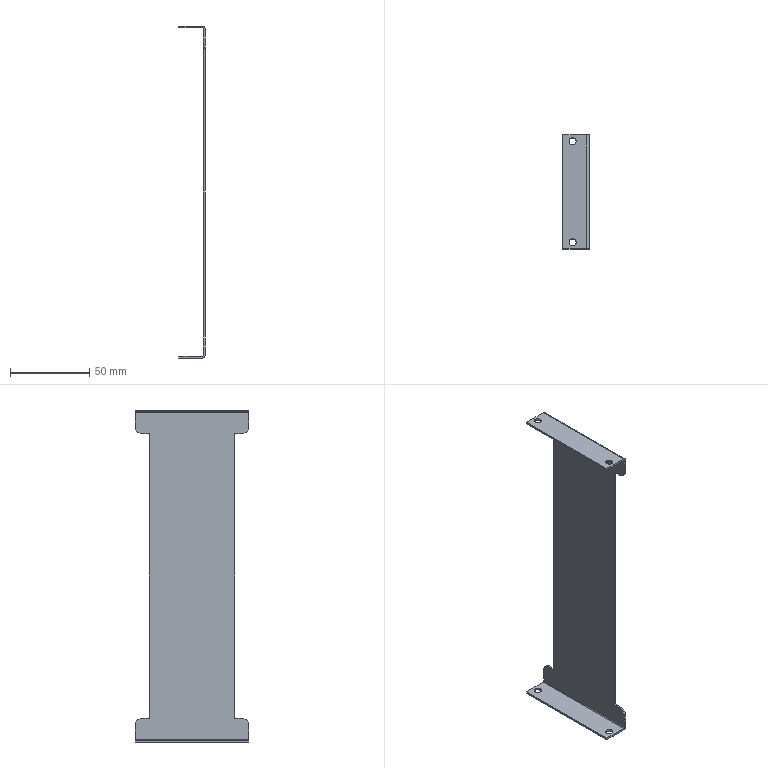Part | STEP file | 复件 FFH80-GY-007^复件 FFH85-B3 -02_三轴模组 | 1 solid | 34 faces | box 16.7 x 71.8 x 210 mm | volume 16698 mm3 | plane 18 | cylinder 16 | commonest cylinder face diameters 4.5 x8 8 x4 1 x2 3.4 x2
STEP:
#1=CARTESIAN_POINT('',(-12.75,-32.,102.6));
#2=VERTEX_POINT('',#1);
#3=CARTESIAN_POINT('',(-8.25,-32.,102.6));
#4=VERTEX_POINT('',#3);
#5=CARTESIAN_POINT('',(-10.5,-32.,102.6));
#6=DIRECTION('',(0.,0.,1.));
#7=DIRECTION('',(1.,0.,0.));
#8=AXIS2_PLACEMENT_3D('',#5,#6,#7);
#9=CIRCLE('',#8,2.25);
#10=EDGE_CURVE('',#2,#4,#9,.T.);
#11=ORIENTED_EDGE('',*,*,#10,.F.);
#12=CARTESIAN_POINT('',(-12.75,-32.,103.8));
#13=VERTEX_POINT('',#12);
#14=CARTESIAN_POINT('',(-12.75,-32.,-106.2));
#15=DIRECTION('',(0.,0.,1.));
#16=VECTOR('',#15,1000.);
#17=LINE('',#14,#16);
#18=EDGE_CURVE('',#2,#13,#17,.T.);
#19=ORIENTED_EDGE('',*,*,#18,.T.);
#20=CARTESIAN_POINT('',(-8.25,-32.,103.8));
#21=VERTEX_POINT('',#20);
#22=CARTESIAN_POINT('',(-10.5,-32.,103.8));
#23=DIRECTION('',(0.,0.,1.));
#24=DIRECTION('',(1.,0.,0.));
#25=AXIS2_PLACEMENT_3D('',#22,#23,#24);
#26=CIRCLE('',#25,2.25);
#27=EDGE_CURVE('',#13,#21,#26,.T.);
#28=ORIENTED_EDGE('',*,*,#27,.T.);
#29=CARTESIAN_POINT('',(-8.25,-32.,-106.2));
#30=DIRECTION('',(0.,0.,1.));
#31=VECTOR('',#30,1000.);
#32=LINE('',#29,#31);
#33=EDGE_CURVE('',#4,#21,#32,.T.);
#34=ORIENTED_EDGE('',*,*,#33,.F.);
#35=EDGE_LOOP('',(#11,#19,#28,#34));
#36=FACE_OUTER_BOUND('',#35,.T.);
#37=CARTESIAN_POINT('',(-10.5,-32.,-106.2));
#38=DIRECTION('',(0.,0.,1.));
#39=DIRECTION('',(1.,0.,0.));
#40=AXIS2_PLACEMENT_3D('',#37,#38,#39);
#41=CYLINDRICAL_SURFACE('',#40,2.25);
#42=ADVANCED_FACE('',(#36),#41,.F.);
#43=CARTESIAN_POINT('',(-12.75,32.,102.6));
#44=VERTEX_POINT('',#43);
#45=CARTESIAN_POINT('',(-8.25,32.,102.6));
#46=VERTEX_POINT('',#45);
#47=CARTESIAN_POINT('',(-10.5,32.,102.6));
#48=DIRECTION('',(0.,0.,1.));
#49=DIRECTION('',(1.,0.,0.));
#50=AXIS2_PLACEMENT_3D('',#47,#48,#49);
#51=CIRCLE('',#50,2.25);
#52=EDGE_CURVE('',#44,#46,#51,.T.);
#53=ORIENTED_EDGE('',*,*,#52,.F.);
#54=CARTESIAN_POINT('',(-12.75,32.,103.8));
#55=VERTEX_POINT('',#54);
#56=CARTESIAN_POINT('',(-12.75,32.,-106.2));
#57=DIRECTION('',(0.,0.,1.));
#58=VECTOR('',#57,1000.);
#59=LINE('',#56,#58);
#60=EDGE_CURVE('',#44,#55,#59,.T.);
#61=ORIENTED_EDGE('',*,*,#60,.T.);
#62=CARTESIAN_POINT('',(-8.25,32.,103.8));
#63=VERTEX_POINT('',#62);
#64=CARTESIAN_POINT('',(-10.5,32.,103.8));
#65=DIRECTION('',(0.,0.,1.));
#66=DIRECTION('',(1.,0.,0.));
#67=AXIS2_PLACEMENT_3D('',#64,#65,#66);
#68=CIRCLE('',#67,2.25);
#69=EDGE_CURVE('',#55,#63,#68,.T.);
#70=ORIENTED_EDGE('',*,*,#69,.T.);
#71=CARTESIAN_POINT('',(-8.25,32.,-106.2));
#72=DIRECTION('',(0.,0.,1.));
#73=VECTOR('',#72,1000.);
#74=LINE('',#71,#73);
#75=EDGE_CURVE('',#46,#63,#74,.T.);
#76=ORIENTED_EDGE('',*,*,#75,.F.);
#77=EDGE_LOOP('',(#53,#61,#70,#76));
#78=FACE_OUTER_BOUND('',#77,.T.);
#79=CARTESIAN_POINT('',(-10.5,32.,-106.2));
#80=DIRECTION('',(0.,0.,1.));
#81=DIRECTION('',(1.,0.,0.));
#82=AXIS2_PLACEMENT_3D('',#79,#80,#81);
#83=CYLINDRICAL_SURFACE('',#82,2.25);
#84=ADVANCED_FACE('',(#78),#83,.F.);
#85=CARTESIAN_POINT('',(-8.25,-32.,-106.2));
#86=VERTEX_POINT('',#85);
#87=CARTESIAN_POINT('',(-12.75,-32.,-106.2));
#88=VERTEX_POINT('',#87);
#89=CARTESIAN_POINT('',(-10.5,-32.,-106.2));
#90=DIRECTION('',(0.,0.,-1.));
#91=DIRECTION('',(1.,0.,0.));
#92=AXIS2_PLACEMENT_3D('',#89,#90,#91);
#93=CIRCLE('',#92,2.25);
#94=EDGE_CURVE('',#86,#88,#93,.T.);
#95=ORIENTED_EDGE('',*,*,#94,.T.);
#96=CARTESIAN_POINT('',(-12.75,-32.,-105.));
#97=VERTEX_POINT('',#96);
#98=CARTESIAN_POINT('',(-12.75,-32.,-106.2));
#99=DIRECTION('',(0.,0.,1.));
#100=VECTOR('',#99,1000.);
#101=LINE('',#98,#100);
#102=EDGE_CURVE('',#88,#97,#101,.T.);
#103=ORIENTED_EDGE('',*,*,#102,.T.);
#104=CARTESIAN_POINT('',(-8.25,-32.,-105.));
#105=VERTEX_POINT('',#104);
#106=CARTESIAN_POINT('',(-10.5,-32.,-105.));
#107=DIRECTION('',(0.,0.,-1.));
#108=DIRECTION('',(1.,0.,0.));
#109=AXIS2_PLACEMENT_3D('',#106,#107,#108);
#110=CIRCLE('',#109,2.25);
#111=EDGE_CURVE('',#105,#97,#110,.T.);
#112=ORIENTED_EDGE('',*,*,#111,.F.);
#113=CARTESIAN_POINT('',(-8.25,-32.,-106.2));
#114=DIRECTION('',(0.,0.,1.));
#115=VECTOR('',#114,1000.);
#116=LINE('',#113,#115);
#117=EDGE_CURVE('',#86,#105,#116,.T.);
#118=ORIENTED_EDGE('',*,*,#117,.F.);
#119=EDGE_LOOP('',(#95,#103,#112,#118));
#120=FACE_OUTER_BOUND('',#119,.T.);
#121=CARTESIAN_POINT('',(-10.5,-32.,-106.2));
#122=DIRECTION('',(0.,0.,1.));
#123=DIRECTION('',(1.,0.,0.));
#124=AXIS2_PLACEMENT_3D('',#121,#122,#123);
#125=CYLINDRICAL_SURFACE('',#124,2.25);
#126=ADVANCED_FACE('',(#120),#125,.F.);
#127=CARTESIAN_POINT('',(-8.25,32.,-106.2));
#128=VERTEX_POINT('',#127);
#129=CARTESIAN_POINT('',(-12.75,32.,-106.2));
#130=VERTEX_POINT('',#129);
#131=CARTESIAN_POINT('',(-10.5,32.,-106.2));
#132=DIRECTION('',(0.,0.,-1.));
#133=DIRECTION('',(1.,0.,0.));
#134=AXIS2_PLACEMENT_3D('',#131,#132,#133);
#135=CIRCLE('',#134,2.25);
#136=EDGE_CURVE('',#128,#130,#135,.T.);
#137=ORIENTED_EDGE('',*,*,#136,.T.);
#138=CARTESIAN_POINT('',(-12.75,32.,-105.));
#139=VERTEX_POINT('',#138);
#140=CARTESIAN_POINT('',(-12.75,32.,-106.2));
#141=DIRECTION('',(0.,0.,1.));
#142=VECTOR('',#141,1000.);
#143=LINE('',#140,#142);
#144=EDGE_CURVE('',#130,#139,#143,.T.);
#145=ORIENTED_EDGE('',*,*,#144,.T.);
#146=CARTESIAN_POINT('',(-8.25,32.,-105.));
#147=VERTEX_POINT('',#146);
#148=CARTESIAN_POINT('',(-10.5,32.,-105.));
#149=DIRECTION('',(0.,0.,-1.));
#150=DIRECTION('',(1.,0.,0.));
#151=AXIS2_PLACEMENT_3D('',#148,#149,#150);
#152=CIRCLE('',#151,2.25);
#153=EDGE_CURVE('',#147,#139,#152,.T.);
#154=ORIENTED_EDGE('',*,*,#153,.F.);
#155=CARTESIAN_POINT('',(-8.25,32.,-106.2));
#156=DIRECTION('',(0.,0.,1.));
#157=VECTOR('',#156,1000.);
#158=LINE('',#155,#157);
#159=EDGE_CURVE('',#128,#147,#158,.T.);
#160=ORIENTED_EDGE('',*,*,#159,.F.);
#161=EDGE_LOOP('',(#137,#145,#154,#160));
#162=FACE_OUTER_BOUND('',#161,.T.);
#163=CARTESIAN_POINT('',(-10.5,32.,-106.2));
#164=DIRECTION('',(0.,0.,1.));
#165=DIRECTION('',(1.,0.,0.));
#166=AXIS2_PLACEMENT_3D('',#163,#164,#165);
#167=CYLINDRICAL_SURFACE('',#166,2.25);
#168=ADVANCED_FACE('',(#162),#167,.F.);
#169=CARTESIAN_POINT('',(0.,-35.9,102.1));
#170=VERTEX_POINT('',#169);
#171=CARTESIAN_POINT('',(0.,-35.9,92.9));
#172=VERTEX_POINT('',#171);
#173=CARTESIAN_POINT('',(0.,-35.9,0.));
#174=DIRECTION('',(0.,0.,-1.));
#175=VECTOR('',#174,1000.);
#176=LINE('',#173,#175);
#177=EDGE_CURVE('',#170,#172,#176,.T.);
#178=ORIENTED_EDGE('',*,*,#177,.T.);
#179=CARTESIAN_POINT('',(0.,-31.9,88.9));
#180=VERTEX_POINT('',#179);
#181=CARTESIAN_POINT('',(0.,-31.9,92.9));
#182=DIRECTION('',(1.,0.,0.));
#183=DIRECTION('',(0.,0.,-1.));
#184=AXIS2_PLACEMENT_3D('',#181,#182,#183);
#185=CIRCLE('',#184,4.);
#186=EDGE_CURVE('',#172,#180,#185,.T.);
#187=ORIENTED_EDGE('',*,*,#186,.T.);
#188=CARTESIAN_POINT('',(0.,-26.9,88.9));
#189=VERTEX_POINT('',#188);
#190=CARTESIAN_POINT('',(0.,0.,88.9));
#191=DIRECTION('',(0.,1.,0.));
#192=VECTOR('',#191,1000.);
#193=LINE('',#190,#192);
#194=EDGE_CURVE('',#180,#189,#193,.T.);
#195=ORIENTED_EDGE('',*,*,#194,.T.);
#196=CARTESIAN_POINT('',(0.,-26.9,-91.3));
#197=VERTEX_POINT('',#196);
#198=CARTESIAN_POINT('',(0.,-26.9,0.));
#199=DIRECTION('',(0.,0.,-1.));
#200=VECTOR('',#199,1000.);
#201=LINE('',#198,#200);
#202=EDGE_CURVE('',#189,#197,#201,.T.);
#203=ORIENTED_EDGE('',*,*,#202,.T.);
#204=CARTESIAN_POINT('',(0.,-31.9,-91.3));
#205=VERTEX_POINT('',#204);
#206=CARTESIAN_POINT('',(0.,0.,-91.3));
#207=DIRECTION('',(0.,-1.,0.));
#208=VECTOR('',#207,1000.);
#209=LINE('',#206,#208);
#210=EDGE_CURVE('',#197,#205,#209,.T.);
#211=ORIENTED_EDGE('',*,*,#210,.T.);
#212=CARTESIAN_POINT('',(0.,-35.9,-95.3));
#213=VERTEX_POINT('',#212);
#214=CARTESIAN_POINT('',(0.,-31.9,-95.3));
#215=DIRECTION('',(1.,0.,0.));
#216=DIRECTION('',(0.,0.,-1.));
#217=AXIS2_PLACEMENT_3D('',#214,#215,#216);
#218=CIRCLE('',#217,4.);
#219=EDGE_CURVE('',#205,#213,#218,.T.);
#220=ORIENTED_EDGE('',*,*,#219,.T.);
#221=CARTESIAN_POINT('',(0.,-35.9,-104.5));
#222=VERTEX_POINT('',#221);
#223=CARTESIAN_POINT('',(0.,-35.9,0.));
#224=DIRECTION('',(0.,0.,-1.));
#225=VECTOR('',#224,1000.);
#226=LINE('',#223,#225);
#227=EDGE_CURVE('',#213,#222,#226,.T.);
#228=ORIENTED_EDGE('',*,*,#227,.T.);
#229=CARTESIAN_POINT('',(0.,35.9,-104.5));
#230=VERTEX_POINT('',#229);
#231=CARTESIAN_POINT('',(0.,0.,-104.5));
#232=DIRECTION('',(0.,1.,0.));
#233=VECTOR('',#232,1000.);
#234=LINE('',#231,#233);
#235=EDGE_CURVE('',#222,#230,#234,.T.);
#236=ORIENTED_EDGE('',*,*,#235,.T.);
#237=CARTESIAN_POINT('',(0.,35.9,-95.3));
#238=VERTEX_POINT('',#237);
#239=CARTESIAN_POINT('',(0.,35.9,0.));
#240=DIRECTION('',(0.,0.,1.));
#241=VECTOR('',#240,1000.);
#242=LINE('',#239,#241);
#243=EDGE_CURVE('',#230,#238,#242,.T.);
#244=ORIENTED_EDGE('',*,*,#243,.T.);
#245=CARTESIAN_POINT('',(0.,31.9,-91.3));
#246=VERTEX_POINT('',#245);
#247=CARTESIAN_POINT('',(0.,31.9,-95.3));
#248=DIRECTION('',(1.,0.,0.));
#249=DIRECTION('',(0.,0.,-1.));
#250=AXIS2_PLACEMENT_3D('',#247,#248,#249);
#251=CIRCLE('',#250,4.);
#252=EDGE_CURVE('',#238,#246,#251,.T.);
#253=ORIENTED_EDGE('',*,*,#252,.T.);
#254=CARTESIAN_POINT('',(0.,26.9,-91.3));
#255=VERTEX_POINT('',#254);
#256=CARTESIAN_POINT('',(0.,0.,-91.3));
#257=DIRECTION('',(0.,-1.,0.));
#258=VECTOR('',#257,1000.);
#259=LINE('',#256,#258);
#260=EDGE_CURVE('',#246,#255,#259,.T.);
#261=ORIENTED_EDGE('',*,*,#260,.T.);
#262=CARTESIAN_POINT('',(0.,26.9,88.9));
#263=VERTEX_POINT('',#262);
#264=CARTESIAN_POINT('',(0.,26.9,0.));
#265=DIRECTION('',(0.,0.,1.));
#266=VECTOR('',#265,1000.);
#267=LINE('',#264,#266);
#268=EDGE_CURVE('',#255,#263,#267,.T.);
#269=ORIENTED_EDGE('',*,*,#268,.T.);
#270=CARTESIAN_POINT('',(0.,31.9,88.9));
#271=VERTEX_POINT('',#270);
#272=CARTESIAN_POINT('',(0.,0.,88.9));
#273=DIRECTION('',(0.,1.,0.));
#274=VECTOR('',#273,1000.);
#275=LINE('',#272,#274);
#276=EDGE_CURVE('',#263,#271,#275,.T.);
#277=ORIENTED_EDGE('',*,*,#276,.T.);
#278=CARTESIAN_POINT('',(0.,35.9,92.9));
#279=VERTEX_POINT('',#278);
#280=CARTESIAN_POINT('',(0.,31.9,92.9));
#281=DIRECTION('',(1.,0.,0.));
#282=DIRECTION('',(0.,0.,-1.));
#283=AXIS2_PLACEMENT_3D('',#280,#281,#282);
#284=CIRCLE('',#283,4.);
#285=EDGE_CURVE('',#271,#279,#284,.T.);
#286=ORIENTED_EDGE('',*,*,#285,.T.);
#287=CARTESIAN_POINT('',(0.,35.9,102.1));
#288=VERTEX_POINT('',#287);
#289=CARTESIAN_POINT('',(0.,35.9,0.));
#290=DIRECTION('',(0.,0.,1.));
#291=VECTOR('',#290,1000.);
#292=LINE('',#289,#291);
#293=EDGE_CURVE('',#279,#288,#292,.T.);
#294=ORIENTED_EDGE('',*,*,#293,.T.);
#295=CARTESIAN_POINT('',(0.,0.,102.1));
#296=DIRECTION('',(0.,-1.,0.));
#297=VECTOR('',#296,1000.);
#298=LINE('',#295,#297);
#299=EDGE_CURVE('',#288,#170,#298,.T.);
#300=ORIENTED_EDGE('',*,*,#299,.T.);
#301=EDGE_LOOP('',(#178,#187,#195,#203,#211,#220,#228,#236,#244,#253,#261,#269,#277,#286,#294,#300));
#302=FACE_OUTER_BOUND('',#301,.T.);
#303=CARTESIAN_POINT('',(0.,0.,0.));
#304=DIRECTION('',(1.,0.,0.));
#305=DIRECTION('',(0.,0.,-1.));
#306=AXIS2_PLACEMENT_3D('',#303,#304,#305);
#307=PLANE('',#306);
#308=ADVANCED_FACE('',(#302),#307,.T.);
#309=CARTESIAN_POINT('',(-1.2,-35.9,92.9));
#310=VERTEX_POINT('',#309);
#311=CARTESIAN_POINT('',(-1.2,-31.9,88.9));
#312=VERTEX_POINT('',#311);
#313=CARTESIAN_POINT('',(-1.2,-31.9,92.9));
#314=DIRECTION('',(1.,0.,0.));
#315=DIRECTION('',(0.,0.,-1.));
#316=AXIS2_PLACEMENT_3D('',#313,#314,#315);
#317=CIRCLE('',#316,4.);
#318=EDGE_CURVE('',#310,#312,#317,.T.);
#319=ORIENTED_EDGE('',*,*,#318,.T.);
#320=CARTESIAN_POINT('',(-1.2,-31.9,88.9));
#321=DIRECTION('',(1.,0.,0.));
#322=VECTOR('',#321,1000.);
#323=LINE('',#320,#322);
#324=EDGE_CURVE('',#312,#180,#323,.T.);
#325=ORIENTED_EDGE('',*,*,#324,.T.);
#326=ORIENTED_EDGE('',*,*,#186,.F.);
#327=CARTESIAN_POINT('',(-1.2,-35.9,92.9));
#328=DIRECTION('',(-1.,0.,0.));
#329=VECTOR('',#328,1000.);
#330=LINE('',#327,#329);
#331=EDGE_CURVE('',#172,#310,#330,.T.);
#332=ORIENTED_EDGE('',*,*,#331,.T.);
#333=EDGE_LOOP('',(#319,#325,#326,#332));
#334=FACE_OUTER_BOUND('',#333,.T.);
#335=CARTESIAN_POINT('',(-1.2,-31.9,92.9));
#336=DIRECTION('',(1.,0.,0.));
#337=DIRECTION('',(0.,0.,-1.));
#338=AXIS2_PLACEMENT_3D('',#335,#336,#337);
#339=CYLINDRICAL_SURFACE('',#338,4.);
#340=ADVANCED_FACE('',(#334),#339,.T.);
#341=CARTESIAN_POINT('',(-1.2,-35.9,102.1));
#342=VERTEX_POINT('',#341);
#343=CARTESIAN_POINT('',(-1.2,-35.9,88.9));
#344=DIRECTION('',(0.,0.,-1.));
#345=VECTOR('',#344,1000.);
#346=LINE('',#343,#345);
#347=EDGE_CURVE('',#342,#310,#346,.T.);
#348=ORIENTED_EDGE('',*,*,#347,.T.);
#349=ORIENTED_EDGE('',*,*,#331,.F.);
#350=ORIENTED_EDGE('',*,*,#177,.F.);
#351=CARTESIAN_POINT('',(-1.7,-35.9,103.8));
#352=VERTEX_POINT('',#351);
#353=CARTESIAN_POINT('',(-1.7,-35.9,102.1));
#354=DIRECTION('',(0.,-1.,0.));
#355=DIRECTION('',(0.,0.,1.));
#356=AXIS2_PLACEMENT_3D('',#353,#354,#355);
#357=CIRCLE('',#356,1.7);
#358=EDGE_CURVE('',#170,#352,#357,.T.);
#359=ORIENTED_EDGE('',*,*,#358,.T.);
#360=CARTESIAN_POINT('',(-16.7,-35.9,103.8));
#361=VERTEX_POINT('',#360);
#362=CARTESIAN_POINT('',(-1.2,-35.9,103.8));
#363=DIRECTION('',(-1.,0.,0.));
#364=VECTOR('',#363,1000.);
#365=LINE('',#362,#364);
#366=EDGE_CURVE('',#352,#361,#365,.T.);
#367=ORIENTED_EDGE('',*,*,#366,.T.);
#368=CARTESIAN_POINT('',(-16.7,-35.9,102.6));
#369=VERTEX_POINT('',#368);
#370=CARTESIAN_POINT('',(-16.7,-35.9,103.8));
#371=DIRECTION('',(0.,0.,-1.));
#372=VECTOR('',#371,1000.);
#373=LINE('',#370,#372);
#374=EDGE_CURVE('',#361,#369,#373,.T.);
#375=ORIENTED_EDGE('',*,*,#374,.T.);
#376=CARTESIAN_POINT('',(-1.7,-35.9,102.6));
#377=VERTEX_POINT('',#376);
#378=CARTESIAN_POINT('',(-1.2,-35.9,102.6));
#379=DIRECTION('',(1.,0.,0.));
#380=VECTOR('',#379,1000.);
#381=LINE('',#378,#380);
#382=EDGE_CURVE('',#369,#377,#381,.T.);
#383=ORIENTED_EDGE('',*,*,#382,.T.);
#384=CARTESIAN_POINT('',(-1.7,-35.9,102.1));
#385=DIRECTION('',(0.,1.,0.));
#386=DIRECTION('',(0.,0.,1.));
#387=AXIS2_PLACEMENT_3D('',#384,#385,#386);
#388=CIRCLE('',#387,0.5);
#389=EDGE_CURVE('',#377,#342,#388,.T.);
#390=ORIENTED_EDGE('',*,*,#389,.T.);
#391=EDGE_LOOP('',(#348,#349,#350,#359,#367,#375,#383,#390));
#392=FACE_OUTER_BOUND('',#391,.T.);
#393=CARTESIAN_POINT('',(-1.2,-35.9,88.9));
#394=DIRECTION('',(0.,-1.,0.));
#395=DIRECTION('',(0.,0.,-1.));
#396=AXIS2_PLACEMENT_3D('',#393,#394,#395);
#397=PLANE('',#396);
#398=ADVANCED_FACE('',(#392),#397,.T.);
#399=ORIENTED_EDGE('',*,*,#299,.F.);
#400=CARTESIAN_POINT('',(-1.7,35.9,103.8));
#401=VERTEX_POINT('',#400);
#402=CARTESIAN_POINT('',(-1.7,35.9,102.1));
#403=DIRECTION('',(0.,-1.,0.));
#404=DIRECTION('',(0.,0.,1.));
#405=AXIS2_PLACEMENT_3D('',#402,#403,#404);
#406=CIRCLE('',#405,1.7);
#407=EDGE_CURVE('',#288,#401,#406,.T.);
#408=ORIENTED_EDGE('',*,*,#407,.T.);
#409=CARTESIAN_POINT('',(-1.7,35.9,103.8));
#410=DIRECTION('',(0.,-1.,0.));
#411=VECTOR('',#410,1000.);
#412=LINE('',#409,#411);
#413=EDGE_CURVE('',#401,#352,#412,.T.);
#414=ORIENTED_EDGE('',*,*,#413,.T.);
#415=ORIENTED_EDGE('',*,*,#358,.F.);
#416=EDGE_LOOP('',(#399,#408,#414,#415));
#417=FACE_OUTER_BOUND('',#416,.T.);
#418=CARTESIAN_POINT('',(-1.7,35.9,102.1));
#419=DIRECTION('',(0.,1.,0.));
#420=DIRECTION('',(0.,0.,1.));
#421=AXIS2_PLACEMENT_3D('',#418,#419,#420);
#422=CYLINDRICAL_SURFACE('',#421,1.7);
#423=ADVANCED_FACE('',(#417),#422,.T.);
#424=ORIENTED_EDGE('',*,*,#293,.F.);
#425=CARTESIAN_POINT('',(-1.2,35.9,92.9));
#426=VERTEX_POINT('',#425);
#427=CARTESIAN_POINT('',(-1.2,35.9,92.9));
#428=DIRECTION('',(-1.,0.,0.));
#429=VECTOR('',#428,1000.);
#430=LINE('',#427,#429);
#431=EDGE_CURVE('',#279,#426,#430,.T.);
#432=ORIENTED_EDGE('',*,*,#431,.T.);
#433=CARTESIAN_POINT('',(-1.2,35.9,102.1));
#434=VERTEX_POINT('',#433);
#435=CARTESIAN_POINT('',(-1.2,35.9,88.9));
#436=DIRECTION('',(0.,0.,1.));
#437=VECTOR('',#436,1000.);
#438=LINE('',#435,#437);
#439=EDGE_CURVE('',#426,#434,#438,.T.);
#440=ORIENTED_EDGE('',*,*,#439,.T.);
#441=CARTESIAN_POINT('',(-1.7,35.9,102.6));
#442=VERTEX_POINT('',#441);
#443=CARTESIAN_POINT('',(-1.7,35.9,102.1));
#444=DIRECTION('',(0.,-1.,0.));
#445=DIRECTION('',(0.,0.,1.));
#446=AXIS2_PLACEMENT_3D('',#443,#444,#445);
#447=CIRCLE('',#446,0.5);
#448=EDGE_CURVE('',#434,#442,#447,.T.);
#449=ORIENTED_EDGE('',*,*,#448,.T.);
#450=CARTESIAN_POINT('',(-16.7,35.9,102.6));
#451=VERTEX_POINT('',#450);
#452=CARTESIAN_POINT('',(-1.2,35.9,102.6));
#453=DIRECTION('',(-1.,0.,0.));
#454=VECTOR('',#453,1000.);
#455=LINE('',#452,#454);
#456=EDGE_CURVE('',#442,#451,#455,.T.);
#457=ORIENTED_EDGE('',*,*,#456,.T.);
#458=CARTESIAN_POINT('',(-16.7,35.9,103.8));
#459=VERTEX_POINT('',#458);
#460=CARTESIAN_POINT('',(-16.7,35.9,103.8));
#461=DIRECTION('',(0.,0.,1.));
#462=VECTOR('',#461,1000.);
#463=LINE('',#460,#462);
#464=EDGE_CURVE('',#451,#459,#463,.T.);
#465=ORIENTED_EDGE('',*,*,#464,.T.);
#466=CARTESIAN_POINT('',(-1.2,35.9,103.8));
#467=DIRECTION('',(1.,0.,0.));
#468=VECTOR('',#467,1000.);
#469=LINE('',#466,#468);
#470=EDGE_CURVE('',#459,#401,#469,.T.);
#471=ORIENTED_EDGE('',*,*,#470,.T.);
#472=ORIENTED_EDGE('',*,*,#407,.F.);
#473=EDGE_LOOP('',(#424,#432,#440,#449,#457,#465,#471,#472));
#474=FACE_OUTER_BOUND('',#473,.T.);
#475=CARTESIAN_POINT('',(-1.2,35.9,88.9));
#476=DIRECTION('',(0.,1.,0.));
#477=DIRECTION('',(0.,0.,1.));
#478=AXIS2_PLACEMENT_3D('',#475,#476,#477);
#479=PLANE('',#478);
#480=ADVANCED_FACE('',(#474),#479,.T.);
#481=CARTESIAN_POINT('',(-1.2,31.9,88.9));
#482=VERTEX_POINT('',#481);
#483=CARTESIAN_POINT('',(-1.2,31.9,92.9));
#484=DIRECTION('',(1.,0.,0.));
#485=DIRECTION('',(0.,0.,-1.));
#486=AXIS2_PLACEMENT_3D('',#483,#484,#485);
#487=CIRCLE('',#486,4.);
#488=EDGE_CURVE('',#482,#426,#487,.T.);
#489=ORIENTED_EDGE('',*,*,#488,.T.);
#490=ORIENTED_EDGE('',*,*,#431,.F.);
#491=ORIENTED_EDGE('',*,*,#285,.F.);
#492=CARTESIAN_POINT('',(-1.2,31.9,88.9));
#493=DIRECTION('',(-1.,0.,0.));
#494=VECTOR('',#493,1000.);
#495=LINE('',#492,#494);
#496=EDGE_CURVE('',#271,#482,#495,.T.);
#497=ORIENTED_EDGE('',*,*,#496,.T.);
#498=EDGE_LOOP('',(#489,#490,#491,#497));
#499=FACE_OUTER_BOUND('',#498,.T.);
#500=CARTESIAN_POINT('',(-1.2,31.9,92.9));
#501=DIRECTION('',(1.,0.,0.));
#502=DIRECTION('',(0.,0.,-1.));
#503=AXIS2_PLACEMENT_3D('',#500,#501,#502);
#504=CYLINDRICAL_SURFACE('',#503,4.);
#505=ADVANCED_FACE('',(#499),#504,.T.);
#506=CARTESIAN_POINT('',(-1.2,26.9,88.9));
#507=VERTEX_POINT('',#506);
#508=CARTESIAN_POINT('',(-1.2,26.9,88.9));
#509=DIRECTION('',(0.,1.,0.));
#510=VECTOR('',#509,1000.);
#511=LINE('',#508,#510);
#512=EDGE_CURVE('',#507,#482,#511,.T.);
#513=ORIENTED_EDGE('',*,*,#512,.T.);
#514=ORIENTED_EDGE('',*,*,#496,.F.);
#515=ORIENTED_EDGE('',*,*,#276,.F.);
#516=CARTESIAN_POINT('',(-1.2,26.9,88.9));
#517=DIRECTION('',(-1.,0.,0.));
#518=VECTOR('',#517,1000.);
#519=LINE('',#516,#518);
#520=EDGE_CURVE('',#263,#507,#519,.T.);
#521=ORIENTED_EDGE('',*,*,#520,.T.);
#522=EDGE_LOOP('',(#513,#514,#515,#521));
#523=FACE_OUTER_BOUND('',#522,.T.);
#524=CARTESIAN_POINT('',(-1.2,26.9,88.9));
#525=DIRECTION('',(0.,0.,-1.));
#526=DIRECTION('',(-1.,0.,0.));
#527=AXIS2_PLACEMENT_3D('',#524,#525,#526);
#528=PLANE('',#527);
#529=ADVANCED_FACE('',(#523),#528,.T.);
#530=ORIENTED_EDGE('',*,*,#268,.F.);
#531=CARTESIAN_POINT('',(-1.2,26.9,-91.3));
#532=VERTEX_POINT('',#531);
#533=CARTESIAN_POINT('',(-1.2,26.9,-91.3));
#534=DIRECTION('',(-1.,0.,0.));
#535=VECTOR('',#534,1000.);
#536=LINE('',#533,#535);
#537=EDGE_CURVE('',#255,#532,#536,.T.);
#538=ORIENTED_EDGE('',*,*,#537,.T.);
#539=CARTESIAN_POINT('',(-1.2,26.9,-91.3));
#540=DIRECTION('',(0.,0.,1.));
#541=VECTOR('',#540,1000.);
#542=LINE('',#539,#541);
#543=EDGE_CURVE('',#532,#507,#542,.T.);
#544=ORIENTED_EDGE('',*,*,#543,.T.);
#545=ORIENTED_EDGE('',*,*,#520,.F.);
#546=EDGE_LOOP('',(#530,#538,#544,#545));
#547=FACE_OUTER_BOUND('',#546,.T.);
#548=CARTESIAN_POINT('',(-1.2,26.9,-91.3));
#549=DIRECTION('',(0.,1.,0.));
#550=DIRECTION('',(0.,0.,1.));
#551=AXIS2_PLACEMENT_3D('',#548,#549,#550);
#552=PLANE('',#551);
#553=ADVANCED_FACE('',(#547),#552,.T.);
#554=ORIENTED_EDGE('',*,*,#260,.F.);
#555=CARTESIAN_POINT('',(-1.2,31.9,-91.3));
#556=VERTEX_POINT('',#555);
#557=CARTESIAN_POINT('',(-1.2,31.9,-91.3));
#558=DIRECTION('',(-1.,0.,0.));
#559=VECTOR('',#558,1000.);
#560=LINE('',#557,#559);
#561=EDGE_CURVE('',#246,#556,#560,.T.);
#562=ORIENTED_EDGE('',*,*,#561,.T.);
#563=CARTESIAN_POINT('',(-1.2,26.9,-91.3));
#564=DIRECTION('',(0.,-1.,0.));
#565=VECTOR('',#564,1000.);
#566=LINE('',#563,#565);
#567=EDGE_CURVE('',#556,#532,#566,.T.);
#568=ORIENTED_EDGE('',*,*,#567,.T.);
#569=ORIENTED_EDGE('',*,*,#537,.F.);
#570=EDGE_LOOP('',(#554,#562,#568,#569));
#571=FACE_OUTER_BOUND('',#570,.T.);
#572=CARTESIAN_POINT('',(-1.2,26.9,-91.3));
#573=DIRECTION('',(0.,0.,1.));
#574=DIRECTION('',(1.,0.,0.));
#575=AXIS2_PLACEMENT_3D('',#572,#573,#574);
#576=PLANE('',#575);
#577=ADVANCED_FACE('',(#571),#576,.T.);
#578=CARTESIAN_POINT('',(-1.2,35.9,-95.3));
#579=VERTEX_POINT('',#578);
#580=CARTESIAN_POINT('',(-1.2,31.9,-95.3));
#581=DIRECTION('',(1.,0.,0.));
#582=DIRECTION('',(0.,0.,-1.));
#583=AXIS2_PLACEMENT_3D('',#580,#581,#582);
#584=CIRCLE('',#583,4.);
#585=EDGE_CURVE('',#579,#556,#584,.T.);
#586=ORIENTED_EDGE('',*,*,#585,.T.);
#587=ORIENTED_EDGE('',*,*,#561,.F.);
#588=ORIENTED_EDGE('',*,*,#252,.F.);
#589=CARTESIAN_POINT('',(-1.2,35.9,-95.3));
#590=DIRECTION('',(-1.,0.,0.));
#591=VECTOR('',#590,1000.);
#592=LINE('',#589,#591);
#593=EDGE_CURVE('',#238,#579,#592,.T.);
#594=ORIENTED_EDGE('',*,*,#593,.T.);
#595=EDGE_LOOP('',(#586,#587,#588,#594));
#596=FACE_OUTER_BOUND('',#595,.T.);
#597=CARTESIAN_POINT('',(-1.2,31.9,-95.3));
#598=DIRECTION('',(1.,0.,0.));
#599=DIRECTION('',(0.,0.,-1.));
#600=AXIS2_PLACEMENT_3D('',#597,#598,#599);
#601=CYLINDRICAL_SURFACE('',#600,4.);
#602=ADVANCED_FACE('',(#596),#601,.T.);
#603=CARTESIAN_POINT('',(-1.2,35.9,-104.5));
#604=VERTEX_POINT('',#603);
#605=CARTESIAN_POINT('',(-1.2,35.9,-91.3));
#606=DIRECTION('',(0.,0.,1.));
#607=VECTOR('',#606,1000.);
#608=LINE('',#605,#607);
#609=EDGE_CURVE('',#604,#579,#608,.T.);
#610=ORIENTED_EDGE('',*,*,#609,.T.);
#611=ORIENTED_EDGE('',*,*,#593,.F.);
#612=ORIENTED_EDGE('',*,*,#243,.F.);
#613=CARTESIAN_POINT('',(-1.7,35.9,-106.2));
#614=VERTEX_POINT('',#613);
#615=CARTESIAN_POINT('',(-1.7,35.9,-104.5));
#616=DIRECTION('',(0.,1.,0.));
#617=DIRECTION('',(0.,0.,-1.));
#618=AXIS2_PLACEMENT_3D('',#615,#616,#617);
#619=CIRCLE('',#618,1.7);
#620=EDGE_CURVE('',#230,#614,#619,.T.);
#621=ORIENTED_EDGE('',*,*,#620,.T.);
#622=CARTESIAN_POINT('',(-16.7,35.9,-106.2));
#623=VERTEX_POINT('',#622);
#624=CARTESIAN_POINT('',(-1.2,35.9,-106.2));
#625=DIRECTION('',(-1.,0.,0.));
#626=VECTOR('',#625,1000.);
#627=LINE('',#624,#626);
#628=EDGE_CURVE('',#614,#623,#627,.T.);
#629=ORIENTED_EDGE('',*,*,#628,.T.);
#630=CARTESIAN_POINT('',(-16.7,35.9,-105.));
#631=VERTEX_POINT('',#630);
#632=CARTESIAN_POINT('',(-16.7,35.9,-106.2));
#633=DIRECTION('',(0.,0.,1.));
#634=VECTOR('',#633,1000.);
#635=LINE('',#632,#634);
#636=EDGE_CURVE('',#623,#631,#635,.T.);
#637=ORIENTED_EDGE('',*,*,#636,.T.);
#638=CARTESIAN_POINT('',(-1.7,35.9,-105.));
#639=VERTEX_POINT('',#638);
#640=CARTESIAN_POINT('',(-1.2,35.9,-105.));
#641=DIRECTION('',(1.,0.,0.));
#642=VECTOR('',#641,1000.);
#643=LINE('',#640,#642);
#644=EDGE_CURVE('',#631,#639,#643,.T.);
#645=ORIENTED_EDGE('',*,*,#644,.T.);
#646=CARTESIAN_POINT('',(-1.7,35.9,-104.5));
#647=DIRECTION('',(0.,-1.,0.));
#648=DIRECTION('',(0.,0.,-1.));
#649=AXIS2_PLACEMENT_3D('',#646,#647,#648);
#650=CIRCLE('',#649,0.5);
#651=EDGE_CURVE('',#639,#604,#650,.T.);
#652=ORIENTED_EDGE('',*,*,#651,.T.);
#653=EDGE_LOOP('',(#610,#611,#612,#621,#629,#637,#645,#652));
#654=FACE_OUTER_BOUND('',#653,.T.);
#655=CARTESIAN_POINT('',(-1.2,35.9,-91.3));
#656=DIRECTION('',(0.,1.,0.));
#657=DIRECTION('',(0.,0.,1.));
#658=AXIS2_PLACEMENT_3D('',#655,#656,#657);
#659=PLANE('',#658);
#660=ADVANCED_FACE('',(#654),#659,.T.);
#661=ORIENTED_EDGE('',*,*,#235,.F.);
#662=CARTESIAN_POINT('',(-1.7,-35.9,-106.2));
#663=VERTEX_POINT('',#662);
#664=CARTESIAN_POINT('',(-1.7,-35.9,-104.5));
#665=DIRECTION('',(0.,1.,0.));
#666=DIRECTION('',(0.,0.,-1.));
#667=AXIS2_PLACEMENT_3D('',#664,#665,#666);
#668=CIRCLE('',#667,1.7);
#669=EDGE_CURVE('',#222,#663,#668,.T.);
#670=ORIENTED_EDGE('',*,*,#669,.T.);
#671=CARTESIAN_POINT('',(-1.7,-35.9,-106.2));
#672=DIRECTION('',(0.,1.,0.));
#673=VECTOR('',#672,1000.);
#674=LINE('',#671,#673);
#675=EDGE_CURVE('',#663,#614,#674,.T.);
#676=ORIENTED_EDGE('',*,*,#675,.T.);
#677=ORIENTED_EDGE('',*,*,#620,.F.);
#678=EDGE_LOOP('',(#661,#670,#676,#677));
#679=FACE_OUTER_BOUND('',#678,.T.);
#680=CARTESIAN_POINT('',(-1.7,-35.9,-104.5));
#681=DIRECTION('',(0.,-1.,0.));
#682=DIRECTION('',(0.,0.,-1.));
#683=AXIS2_PLACEMENT_3D('',#680,#681,#682);
#684=CYLINDRICAL_SURFACE('',#683,1.7);
#685=ADVANCED_FACE('',(#679),#684,.T.);
#686=ORIENTED_EDGE('',*,*,#227,.F.);
#687=CARTESIAN_POINT('',(-1.2,-35.9,-95.3));
#688=VERTEX_POINT('',#687);
#689=CARTESIAN_POINT('',(-1.2,-35.9,-95.3));
#690=DIRECTION('',(-1.,0.,0.));
#691=VECTOR('',#690,1000.);
#692=LINE('',#689,#691);
#693=EDGE_CURVE('',#213,#688,#692,.T.);
#694=ORIENTED_EDGE('',*,*,#693,.T.);
#695=CARTESIAN_POINT('',(-1.2,-35.9,-104.5));
#696=VERTEX_POINT('',#695);
#697=CARTESIAN_POINT('',(-1.2,-35.9,-91.3));
#698=DIRECTION('',(0.,0.,-1.));
#699=VECTOR('',#698,1000.);
#700=LINE('',#697,#699);
#701=EDGE_CURVE('',#688,#696,#700,.T.);
#702=ORIENTED_EDGE('',*,*,#701,.T.);
#703=CARTESIAN_POINT('',(-1.7,-35.9,-105.));
#704=VERTEX_POINT('',#703);
#705=CARTESIAN_POINT('',(-1.7,-35.9,-104.5));
#706=DIRECTION('',(0.,1.,0.));
#707=DIRECTION('',(0.,0.,-1.));
#708=AXIS2_PLACEMENT_3D('',#705,#706,#707);
#709=CIRCLE('',#708,0.5);
#710=EDGE_CURVE('',#696,#704,#709,.T.);
#711=ORIENTED_EDGE('',*,*,#710,.T.);
#712=CARTESIAN_POINT('',(-16.7,-35.9,-105.));
#713=VERTEX_POINT('',#712);
#714=CARTESIAN_POINT('',(-1.2,-35.9,-105.));
#715=DIRECTION('',(-1.,0.,0.));
#716=VECTOR('',#715,1000.);
#717=LINE('',#714,#716);
#718=EDGE_CURVE('',#704,#713,#717,.T.);
#719=ORIENTED_EDGE('',*,*,#718,.T.);
#720=CARTESIAN_POINT('',(-16.7,-35.9,-106.2));
#721=VERTEX_POINT('',#720);
#722=CARTESIAN_POINT('',(-16.7,-35.9,-106.2));
#723=DIRECTION('',(0.,0.,-1.));
#724=VECTOR('',#723,1000.);
#725=LINE('',#722,#724);
#726=EDGE_CURVE('',#713,#721,#725,.T.);
#727=ORIENTED_EDGE('',*,*,#726,.T.);
#728=CARTESIAN_POINT('',(-1.2,-35.9,-106.2));
#729=DIRECTION('',(1.,0.,0.));
#730=VECTOR('',#729,1000.);
#731=LINE('',#728,#730);
#732=EDGE_CURVE('',#721,#663,#731,.T.);
#733=ORIENTED_EDGE('',*,*,#732,.T.);
#734=ORIENTED_EDGE('',*,*,#669,.F.);
#735=EDGE_LOOP('',(#686,#694,#702,#711,#719,#727,#733,#734));
#736=FACE_OUTER_BOUND('',#735,.T.);
#737=CARTESIAN_POINT('',(-1.2,-35.9,-91.3));
#738=DIRECTION('',(0.,-1.,0.));
#739=DIRECTION('',(0.,0.,-1.));
#740=AXIS2_PLACEMENT_3D('',#737,#738,#739);
#741=PLANE('',#740);
#742=ADVANCED_FACE('',(#736),#741,.T.);
#743=CARTESIAN_POINT('',(-1.2,-31.9,-91.3));
#744=VERTEX_POINT('',#743);
#745=CARTESIAN_POINT('',(-1.2,-31.9,-95.3));
#746=DIRECTION('',(1.,0.,0.));
#747=DIRECTION('',(0.,0.,-1.));
#748=AXIS2_PLACEMENT_3D('',#745,#746,#747);
#749=CIRCLE('',#748,4.);
#750=EDGE_CURVE('',#744,#688,#749,.T.);
#751=ORIENTED_EDGE('',*,*,#750,.T.);
#752=ORIENTED_EDGE('',*,*,#693,.F.);
#753=ORIENTED_EDGE('',*,*,#219,.F.);
#754=CARTESIAN_POINT('',(-1.2,-31.9,-91.3));
#755=DIRECTION('',(-1.,0.,0.));
#756=VECTOR('',#755,1000.);
#757=LINE('',#754,#756);
#758=EDGE_CURVE('',#205,#744,#757,.T.);
#759=ORIENTED_EDGE('',*,*,#758,.T.);
#760=EDGE_LOOP('',(#751,#752,#753,#759));
#761=FACE_OUTER_BOUND('',#760,.T.);
#762=CARTESIAN_POINT('',(-1.2,-31.9,-95.3));
#763=DIRECTION('',(1.,0.,0.));
#764=DIRECTION('',(0.,0.,-1.));
#765=AXIS2_PLACEMENT_3D('',#762,#763,#764);
#766=CYLINDRICAL_SURFACE('',#765,4.);
#767=ADVANCED_FACE('',(#761),#766,.T.);
#768=CARTESIAN_POINT('',(-1.2,-26.9,-91.3));
#769=VERTEX_POINT('',#768);
#770=CARTESIAN_POINT('',(-1.2,-26.9,-91.3));
#771=DIRECTION('',(0.,-1.,0.));
#772=VECTOR('',#771,1000.);
#773=LINE('',#770,#772);
#774=EDGE_CURVE('',#769,#744,#773,.T.);
#775=ORIENTED_EDGE('',*,*,#774,.T.);
#776=ORIENTED_EDGE('',*,*,#758,.F.);
#777=ORIENTED_EDGE('',*,*,#210,.F.);
#778=CARTESIAN_POINT('',(-1.2,-26.9,-91.3));
#779=DIRECTION('',(-1.,0.,0.));
#780=VECTOR('',#779,1000.);
#781=LINE('',#778,#780);
#782=EDGE_CURVE('',#197,#769,#781,.T.);
#783=ORIENTED_EDGE('',*,*,#782,.T.);
#784=EDGE_LOOP('',(#775,#776,#777,#783));
#785=FACE_OUTER_BOUND('',#784,.T.);
#786=CARTESIAN_POINT('',(-1.2,-26.9,-91.3));
#787=DIRECTION('',(0.,0.,1.));
#788=DIRECTION('',(1.,0.,0.));
#789=AXIS2_PLACEMENT_3D('',#786,#787,#788);
#790=PLANE('',#789);
#791=ADVANCED_FACE('',(#785),#790,.T.);
#792=ORIENTED_EDGE('',*,*,#202,.F.);
#793=CARTESIAN_POINT('',(-1.2,-26.9,88.9));
#794=VERTEX_POINT('',#793);
#795=CARTESIAN_POINT('',(-1.2,-26.9,88.9));
#796=DIRECTION('',(-1.,0.,0.));
#797=VECTOR('',#796,1000.);
#798=LINE('',#795,#797);
#799=EDGE_CURVE('',#189,#794,#798,.T.);
#800=ORIENTED_EDGE('',*,*,#799,.T.);
#801=CARTESIAN_POINT('',(-1.2,-26.9,-91.3));
#802=DIRECTION('',(0.,0.,-1.));
#803=VECTOR('',#802,1000.);
#804=LINE('',#801,#803);
#805=EDGE_CURVE('',#794,#769,#804,.T.);
#806=ORIENTED_EDGE('',*,*,#805,.T.);
#807=ORIENTED_EDGE('',*,*,#782,.F.);
#808=EDGE_LOOP('',(#792,#800,#806,#807));
#809=FACE_OUTER_BOUND('',#808,.T.);
#810=CARTESIAN_POINT('',(-1.2,-26.9,-91.3));
#811=DIRECTION('',(0.,-1.,0.));
#812=DIRECTION('',(0.,0.,-1.));
#813=AXIS2_PLACEMENT_3D('',#810,#811,#812);
#814=PLANE('',#813);
#815=ADVANCED_FACE('',(#809),#814,.T.);
#816=ORIENTED_EDGE('',*,*,#194,.F.);
#817=ORIENTED_EDGE('',*,*,#324,.F.);
#818=CARTESIAN_POINT('',(-1.2,-26.9,88.9));
#819=DIRECTION('',(0.,1.,0.));
#820=VECTOR('',#819,1000.);
#821=LINE('',#818,#820);
#822=EDGE_CURVE('',#312,#794,#821,.T.);
#823=ORIENTED_EDGE('',*,*,#822,.T.);
#824=ORIENTED_EDGE('',*,*,#799,.F.);
#825=EDGE_LOOP('',(#816,#817,#823,#824));
#826=FACE_OUTER_BOUND('',#825,.T.);
#827=CARTESIAN_POINT('',(-1.2,-26.9,88.9));
#828=DIRECTION('',(0.,0.,-1.));
#829=DIRECTION('',(-1.,0.,0.));
#830=AXIS2_PLACEMENT_3D('',#827,#828,#829);
#831=PLANE('',#830);
#832=ADVANCED_FACE('',(#826),#831,.T.);
#833=ORIENTED_EDGE('',*,*,#774,.F.);
#834=ORIENTED_EDGE('',*,*,#805,.F.);
#835=ORIENTED_EDGE('',*,*,#822,.F.);
#836=ORIENTED_EDGE('',*,*,#318,.F.);
#837=ORIENTED_EDGE('',*,*,#347,.F.);
#838=CARTESIAN_POINT('',(-1.2,0.,102.1));
#839=DIRECTION('',(0.,-1.,0.));
#840=VECTOR('',#839,1000.);
#841=LINE('',#838,#840);
#842=EDGE_CURVE('',#434,#342,#841,.T.);
#843=ORIENTED_EDGE('',*,*,#842,.F.);
#844=ORIENTED_EDGE('',*,*,#439,.F.);
#845=ORIENTED_EDGE('',*,*,#488,.F.);
#846=ORIENTED_EDGE('',*,*,#512,.F.);
#847=ORIENTED_EDGE('',*,*,#543,.F.);
#848=ORIENTED_EDGE('',*,*,#567,.F.);
#849=ORIENTED_EDGE('',*,*,#585,.F.);
#850=ORIENTED_EDGE('',*,*,#609,.F.);
#851=CARTESIAN_POINT('',(-1.2,0.,-104.5));
#852=DIRECTION('',(0.,1.,0.));
#853=VECTOR('',#852,1000.);
#854=LINE('',#851,#853);
#855=EDGE_CURVE('',#696,#604,#854,.T.);
#856=ORIENTED_EDGE('',*,*,#855,.F.);
#857=ORIENTED_EDGE('',*,*,#701,.F.);
#858=ORIENTED_EDGE('',*,*,#750,.F.);
#859=EDGE_LOOP('',(#833,#834,#835,#836,#837,#843,#844,#845,#846,#847,#848,#849,#850,#856,#857,#858));
#860=FACE_OUTER_BOUND('',#859,.T.);
#861=CARTESIAN_POINT('',(-1.2,0.,0.));
#862=DIRECTION('',(1.,0.,0.));
#863=DIRECTION('',(0.,0.,-1.));
#864=AXIS2_PLACEMENT_3D('',#861,#862,#863);
#865=PLANE('',#864);
#866=ADVANCED_FACE('',(#860),#865,.F.);
#867=CARTESIAN_POINT('',(-10.5,-32.,102.6));
#868=DIRECTION('',(0.,0.,1.));
#869=DIRECTION('',(1.,0.,0.));
#870=AXIS2_PLACEMENT_3D('',#867,#868,#869);
#871=CIRCLE('',#870,2.25);
#872=EDGE_CURVE('',#4,#2,#871,.T.);
#873=ORIENTED_EDGE('',*,*,#872,.T.);
#874=ORIENTED_EDGE('',*,*,#10,.T.);
#875=EDGE_LOOP('',(#873,#874));
#876=FACE_BOUND('',#875,.T.);
#877=CARTESIAN_POINT('',(-10.5,32.,102.6));
#878=DIRECTION('',(0.,0.,1.));
#879=DIRECTION('',(1.,0.,0.));
#880=AXIS2_PLACEMENT_3D('',#877,#878,#879);
#881=CIRCLE('',#880,2.25);
#882=EDGE_CURVE('',#46,#44,#881,.T.);
#883=ORIENTED_EDGE('',*,*,#882,.T.);
#884=ORIENTED_EDGE('',*,*,#52,.T.);
#885=EDGE_LOOP('',(#883,#884));
#886=FACE_BOUND('',#885,.T.);
#887=ORIENTED_EDGE('',*,*,#456,.F.);
#888=CARTESIAN_POINT('',(-1.7,0.,102.6));
#889=DIRECTION('',(0.,-1.,0.));
#890=VECTOR('',#889,1000.);
#891=LINE('',#888,#890);
#892=EDGE_CURVE('',#442,#377,#891,.T.);
#893=ORIENTED_EDGE('',*,*,#892,.T.);
#894=ORIENTED_EDGE('',*,*,#382,.F.);
#895=CARTESIAN_POINT('',(-16.7,0.,102.6));
#896=DIRECTION('',(0.,1.,0.));
#897=VECTOR('',#896,1000.);
#898=LINE('',#895,#897);
#899=EDGE_CURVE('',#369,#451,#898,.T.);
#900=ORIENTED_EDGE('',*,*,#899,.T.);
#901=EDGE_LOOP('',(#887,#893,#894,#900));
#902=FACE_OUTER_BOUND('',#901,.T.);
#903=CARTESIAN_POINT('',(0.,0.,102.6));
#904=DIRECTION('',(0.,0.,-1.));
#905=DIRECTION('',(-1.,0.,0.));
#906=AXIS2_PLACEMENT_3D('',#903,#904,#905);
#907=PLANE('',#906);
#908=ADVANCED_FACE('',(#876,#886,#902),#907,.T.);
#909=CARTESIAN_POINT('',(-10.5,-32.,103.8));
#910=DIRECTION('',(0.,0.,1.));
#911=DIRECTION('',(1.,0.,0.));
#912=AXIS2_PLACEMENT_3D('',#909,#910,#911);
#913=CIRCLE('',#912,2.25);
#914=EDGE_CURVE('',#21,#13,#913,.T.);
#915=ORIENTED_EDGE('',*,*,#914,.F.);
#916=ORIENTED_EDGE('',*,*,#27,.F.);
#917=EDGE_LOOP('',(#915,#916));
#918=FACE_BOUND('',#917,.T.);
#919=CARTESIAN_POINT('',(-10.5,32.,103.8));
#920=DIRECTION('',(0.,0.,1.));
#921=DIRECTION('',(1.,0.,0.));
#922=AXIS2_PLACEMENT_3D('',#919,#920,#921);
#923=CIRCLE('',#922,2.25);
#924=EDGE_CURVE('',#63,#55,#923,.T.);
#925=ORIENTED_EDGE('',*,*,#924,.F.);
#926=ORIENTED_EDGE('',*,*,#69,.F.);
#927=EDGE_LOOP('',(#925,#926));
#928=FACE_BOUND('',#927,.T.);
#929=CARTESIAN_POINT('',(-16.7,0.,103.8));
#930=DIRECTION('',(0.,1.,0.));
#931=VECTOR('',#930,1000.);
#932=LINE('',#929,#931);
#933=EDGE_CURVE('',#361,#459,#932,.T.);
#934=ORIENTED_EDGE('',*,*,#933,.F.);
#935=ORIENTED_EDGE('',*,*,#366,.F.);
#936=ORIENTED_EDGE('',*,*,#413,.F.);
#937=ORIENTED_EDGE('',*,*,#470,.F.);
#938=EDGE_LOOP('',(#934,#935,#936,#937));
#939=FACE_OUTER_BOUND('',#938,.T.);
#940=CARTESIAN_POINT('',(0.,0.,103.8));
#941=DIRECTION('',(0.,0.,-1.));
#942=DIRECTION('',(-1.,0.,0.));
#943=AXIS2_PLACEMENT_3D('',#940,#941,#942);
#944=PLANE('',#943);
#945=ADVANCED_FACE('',(#918,#928,#939),#944,.F.);
#946=ORIENTED_EDGE('',*,*,#111,.T.);
#947=CARTESIAN_POINT('',(-10.5,-32.,-105.));
#948=DIRECTION('',(0.,0.,-1.));
#949=DIRECTION('',(1.,0.,0.));
#950=AXIS2_PLACEMENT_3D('',#947,#948,#949);
#951=CIRCLE('',#950,2.25);
#952=EDGE_CURVE('',#97,#105,#951,.T.);
#953=ORIENTED_EDGE('',*,*,#952,.T.);
#954=EDGE_LOOP('',(#946,#953));
#955=FACE_BOUND('',#954,.T.);
#956=ORIENTED_EDGE('',*,*,#153,.T.);
#957=CARTESIAN_POINT('',(-10.5,32.,-105.));
#958=DIRECTION('',(0.,0.,-1.));
#959=DIRECTION('',(1.,0.,0.));
#960=AXIS2_PLACEMENT_3D('',#957,#958,#959);
#961=CIRCLE('',#960,2.25);
#962=EDGE_CURVE('',#139,#147,#961,.T.);
#963=ORIENTED_EDGE('',*,*,#962,.T.);
#964=EDGE_LOOP('',(#956,#963));
#965=FACE_BOUND('',#964,.T.);
#966=ORIENTED_EDGE('',*,*,#718,.F.);
#967=CARTESIAN_POINT('',(-1.7,0.,-105.));
#968=DIRECTION('',(0.,1.,0.));
#969=VECTOR('',#968,1000.);
#970=LINE('',#967,#969);
#971=EDGE_CURVE('',#704,#639,#970,.T.);
#972=ORIENTED_EDGE('',*,*,#971,.T.);
#973=ORIENTED_EDGE('',*,*,#644,.F.);
#974=CARTESIAN_POINT('',(-16.7,0.,-105.));
#975=DIRECTION('',(0.,-1.,0.));
#976=VECTOR('',#975,1000.);
#977=LINE('',#974,#976);
#978=EDGE_CURVE('',#631,#713,#977,.T.);
#979=ORIENTED_EDGE('',*,*,#978,.T.);
#980=EDGE_LOOP('',(#966,#972,#973,#979));
#981=FACE_OUTER_BOUND('',#980,.T.);
#982=CARTESIAN_POINT('',(0.,0.,-105.));
#983=DIRECTION('',(0.,0.,1.));
#984=DIRECTION('',(1.,0.,0.));
#985=AXIS2_PLACEMENT_3D('',#982,#983,#984);
#986=PLANE('',#985);
#987=ADVANCED_FACE('',(#955,#965,#981),#986,.T.);
#988=ORIENTED_EDGE('',*,*,#94,.F.);
#989=CARTESIAN_POINT('',(-10.5,-32.,-106.2));
#990=DIRECTION('',(0.,0.,-1.));
#991=DIRECTION('',(1.,0.,0.));
#992=AXIS2_PLACEMENT_3D('',#989,#990,#991);
#993=CIRCLE('',#992,2.25);
#994=EDGE_CURVE('',#88,#86,#993,.T.);
#995=ORIENTED_EDGE('',*,*,#994,.F.);
#996=EDGE_LOOP('',(#988,#995));
#997=FACE_BOUND('',#996,.T.);
#998=ORIENTED_EDGE('',*,*,#136,.F.);
#999=CARTESIAN_POINT('',(-10.5,32.,-106.2));
#1000=DIRECTION('',(0.,0.,-1.));
#1001=DIRECTION('',(1.,0.,0.));
#1002=AXIS2_PLACEMENT_3D('',#999,#1000,#1001);
#1003=CIRCLE('',#1002,2.25);
#1004=EDGE_CURVE('',#130,#128,#1003,.T.);
#1005=ORIENTED_EDGE('',*,*,#1004,.F.);
#1006=EDGE_LOOP('',(#998,#1005));
#1007=FACE_BOUND('',#1006,.T.);
#1008=CARTESIAN_POINT('',(-16.7,0.,-106.2));
#1009=DIRECTION('',(0.,-1.,0.));
#1010=VECTOR('',#1009,1000.);
#1011=LINE('',#1008,#1010);
#1012=EDGE_CURVE('',#623,#721,#1011,.T.);
#1013=ORIENTED_EDGE('',*,*,#1012,.F.);
#1014=ORIENTED_EDGE('',*,*,#628,.F.);
#1015=ORIENTED_EDGE('',*,*,#675,.F.);
#1016=ORIENTED_EDGE('',*,*,#732,.F.);
#1017=EDGE_LOOP('',(#1013,#1014,#1015,#1016));
#1018=FACE_OUTER_BOUND('',#1017,.T.);
#1019=CARTESIAN_POINT('',(0.,0.,-106.2));
#1020=DIRECTION('',(0.,0.,1.));
#1021=DIRECTION('',(1.,0.,0.));
#1022=AXIS2_PLACEMENT_3D('',#1019,#1020,#1021);
#1023=PLANE('',#1022);
#1024=ADVANCED_FACE('',(#997,#1007,#1018),#1023,.F.);
#1025=ORIENTED_EDGE('',*,*,#892,.F.);
#1026=ORIENTED_EDGE('',*,*,#448,.F.);
#1027=ORIENTED_EDGE('',*,*,#842,.T.);
#1028=ORIENTED_EDGE('',*,*,#389,.F.);
#1029=EDGE_LOOP('',(#1025,#1026,#1027,#1028));
#1030=FACE_OUTER_BOUND('',#1029,.T.);
#1031=CARTESIAN_POINT('',(-1.7,35.9,102.1));
#1032=DIRECTION('',(0.,1.,0.));
#1033=DIRECTION('',(0.,0.,1.));
#1034=AXIS2_PLACEMENT_3D('',#1031,#1032,#1033);
#1035=CYLINDRICAL_SURFACE('',#1034,0.5);
#1036=ADVANCED_FACE('',(#1030),#1035,.F.);
#1037=ORIENTED_EDGE('',*,*,#971,.F.);
#1038=ORIENTED_EDGE('',*,*,#710,.F.);
#1039=ORIENTED_EDGE('',*,*,#855,.T.);
#1040=ORIENTED_EDGE('',*,*,#651,.F.);
#1041=EDGE_LOOP('',(#1037,#1038,#1039,#1040));
#1042=FACE_OUTER_BOUND('',#1041,.T.);
#1043=CARTESIAN_POINT('',(-1.7,-35.9,-104.5));
#1044=DIRECTION('',(0.,-1.,0.));
#1045=DIRECTION('',(0.,0.,-1.));
#1046=AXIS2_PLACEMENT_3D('',#1043,#1044,#1045);
#1047=CYLINDRICAL_SURFACE('',#1046,0.5);
#1048=ADVANCED_FACE('',(#1042),#1047,.F.);
#1049=ORIENTED_EDGE('',*,*,#18,.F.);
#1050=ORIENTED_EDGE('',*,*,#872,.F.);
#1051=ORIENTED_EDGE('',*,*,#33,.T.);
#1052=ORIENTED_EDGE('',*,*,#914,.T.);
#1053=EDGE_LOOP('',(#1049,#1050,#1051,#1052));
#1054=FACE_OUTER_BOUND('',#1053,.T.);
#1055=CARTESIAN_POINT('',(-10.5,-32.,-106.2));
#1056=DIRECTION('',(0.,0.,1.));
#1057=DIRECTION('',(1.,0.,0.));
#1058=AXIS2_PLACEMENT_3D('',#1055,#1056,#1057);
#1059=CYLINDRICAL_SURFACE('',#1058,2.25);
#1060=ADVANCED_FACE('',(#1054),#1059,.F.);
#1061=ORIENTED_EDGE('',*,*,#60,.F.);
#1062=ORIENTED_EDGE('',*,*,#882,.F.);
#1063=ORIENTED_EDGE('',*,*,#75,.T.);
#1064=ORIENTED_EDGE('',*,*,#924,.T.);
#1065=EDGE_LOOP('',(#1061,#1062,#1063,#1064));
#1066=FACE_OUTER_BOUND('',#1065,.T.);
#1067=CARTESIAN_POINT('',(-10.5,32.,-106.2));
#1068=DIRECTION('',(0.,0.,1.));
#1069=DIRECTION('',(1.,0.,0.));
#1070=AXIS2_PLACEMENT_3D('',#1067,#1068,#1069);
#1071=CYLINDRICAL_SURFACE('',#1070,2.25);
#1072=ADVANCED_FACE('',(#1066),#1071,.F.);
#1073=ORIENTED_EDGE('',*,*,#933,.T.);
#1074=ORIENTED_EDGE('',*,*,#464,.F.);
#1075=ORIENTED_EDGE('',*,*,#899,.F.);
#1076=ORIENTED_EDGE('',*,*,#374,.F.);
#1077=EDGE_LOOP('',(#1073,#1074,#1075,#1076));
#1078=FACE_OUTER_BOUND('',#1077,.T.);
#1079=CARTESIAN_POINT('',(-16.7,-35.9,103.8));
#1080=DIRECTION('',(1.,0.,0.));
#1081=DIRECTION('',(0.,0.,-1.));
#1082=AXIS2_PLACEMENT_3D('',#1079,#1080,#1081);
#1083=PLANE('',#1082);
#1084=ADVANCED_FACE('',(#1078),#1083,.F.);
#1085=ORIENTED_EDGE('',*,*,#102,.F.);
#1086=ORIENTED_EDGE('',*,*,#994,.T.);
#1087=ORIENTED_EDGE('',*,*,#117,.T.);
#1088=ORIENTED_EDGE('',*,*,#952,.F.);
#1089=EDGE_LOOP('',(#1085,#1086,#1087,#1088));
#1090=FACE_OUTER_BOUND('',#1089,.T.);
#1091=CARTESIAN_POINT('',(-10.5,-32.,-106.2));
#1092=DIRECTION('',(0.,0.,1.));
#1093=DIRECTION('',(1.,0.,0.));
#1094=AXIS2_PLACEMENT_3D('',#1091,#1092,#1093);
#1095=CYLINDRICAL_SURFACE('',#1094,2.25);
#1096=ADVANCED_FACE('',(#1090),#1095,.F.);
#1097=ORIENTED_EDGE('',*,*,#144,.F.);
#1098=ORIENTED_EDGE('',*,*,#1004,.T.);
#1099=ORIENTED_EDGE('',*,*,#159,.T.);
#1100=ORIENTED_EDGE('',*,*,#962,.F.);
#1101=EDGE_LOOP('',(#1097,#1098,#1099,#1100));
#1102=FACE_OUTER_BOUND('',#1101,.T.);
#1103=CARTESIAN_POINT('',(-10.5,32.,-106.2));
#1104=DIRECTION('',(0.,0.,1.));
#1105=DIRECTION('',(1.,0.,0.));
#1106=AXIS2_PLACEMENT_3D('',#1103,#1104,#1105);
#1107=CYLINDRICAL_SURFACE('',#1106,2.25);
#1108=ADVANCED_FACE('',(#1102),#1107,.F.);
#1109=ORIENTED_EDGE('',*,*,#1012,.T.);
#1110=ORIENTED_EDGE('',*,*,#726,.F.);
#1111=ORIENTED_EDGE('',*,*,#978,.F.);
#1112=ORIENTED_EDGE('',*,*,#636,.F.);
#1113=EDGE_LOOP('',(#1109,#1110,#1111,#1112));
#1114=FACE_OUTER_BOUND('',#1113,.T.);
#1115=CARTESIAN_POINT('',(-16.7,35.9,-106.2));
#1116=DIRECTION('',(1.,0.,0.));
#1117=DIRECTION('',(0.,0.,-1.));
#1118=AXIS2_PLACEMENT_3D('',#1115,#1116,#1117);
#1119=PLANE('',#1118);
#1120=ADVANCED_FACE('',(#1114),#1119,.F.);
#1121=CLOSED_SHELL('',(#42,#84,#126,#168,#308,#340,#398,#423,#480,#505,#529,#553,#577,#602,#660,#685,#742,#767,#791,#815,#832,#866,#908,#945,#987,#1024,#1036,#1048,#1060,#1072,#1084,#1096,#1108,#1120));
#1122=MANIFOLD_SOLID_BREP('',#1121);
#1123=CARTESIAN_POINT('',(0.,0.,0.));
#1124=DIRECTION('',(0.,0.,1.));
#1125=DIRECTION('',(1.,0.,0.));
#1126=AXIS2_PLACEMENT_3D('',#1123,#1124,#1125);
#1127=(LENGTH_UNIT()NAMED_UNIT(*)SI_UNIT(.MILLI.,.METRE.));
#1128=UNCERTAINTY_MEASURE_WITH_UNIT(LENGTH_MEASURE(0.00001),#1127,'','');
#1129=(NAMED_UNIT(*)PLANE_ANGLE_UNIT()SI_UNIT($,.RADIAN.));
#1130=(NAMED_UNIT(*)SI_UNIT($,.STERADIAN.)SOLID_ANGLE_UNIT());
#1131=(GEOMETRIC_REPRESENTATION_CONTEXT(3)GLOBAL_UNCERTAINTY_ASSIGNED_CONTEXT((#1128))GLOBAL_UNIT_ASSIGNED_CONTEXT((#1127,#1129,#1130))REPRESENTATION_CONTEXT('',''));
#1132=ADVANCED_BREP_SHAPE_REPRESENTATION('',(#1122,#1126),#1131);